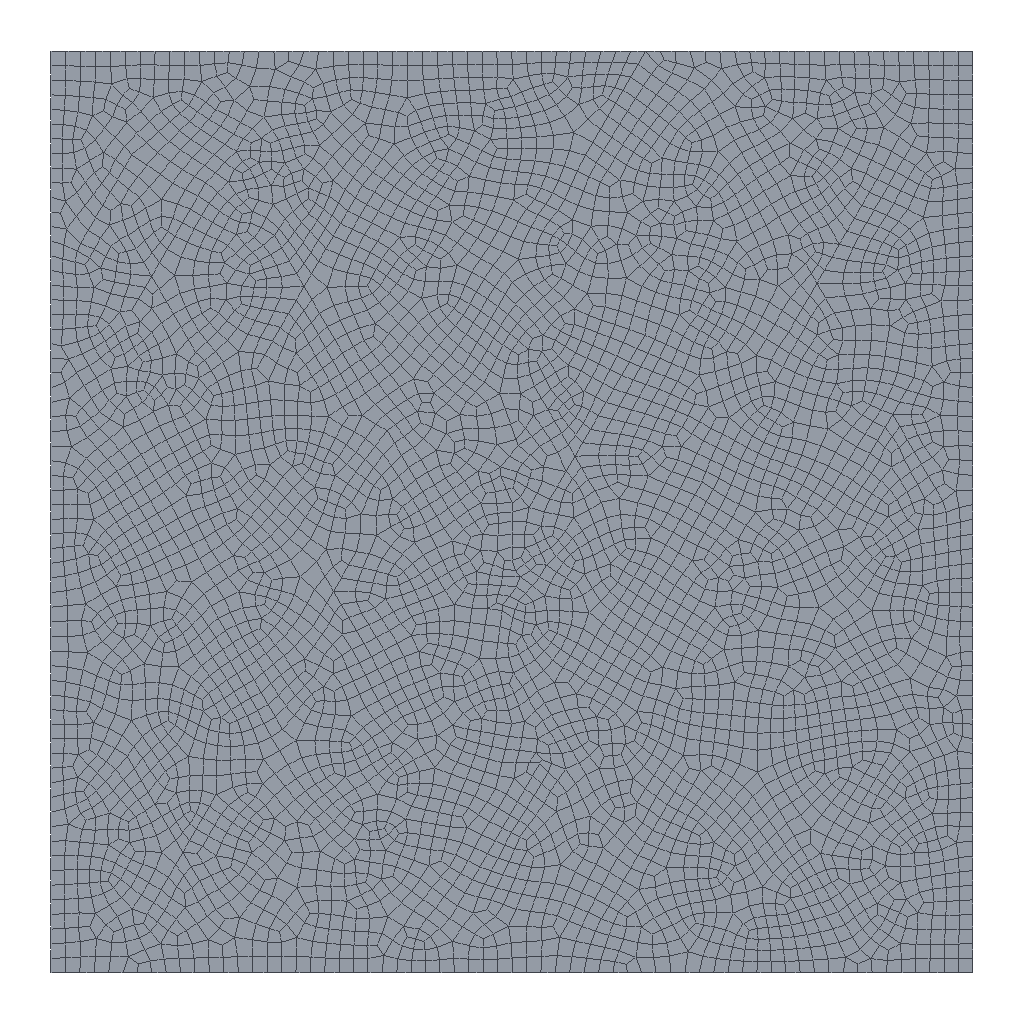Simulation study | abaqus
Notes in the study folder:
模型参数
尺寸 10cm*10cm
预制裂隙如cae
注入位置 和cae文件一样
渗透率 1e-16 m^2
孔隙度 3%
比热容 1.26 kJ/ （kg*K）
热导率 0.25 W/(m·K）
杨氏模量 3000MPa
泊松比 0.35
密度 1.3 g/cm^3

co2流体
 密度 0.5g / cm^3
 粘度 0.000026ps*s
滤失系数 10-3m/min^0.5
温度40℃


注入条件
40ml/min

加载条件
最小水平主应力 11MPa
最大水平主应力  15MPa

温度模型
骨架温度是40℃往中心传导
流体温度是40℃扩展过程中传导
Set-up summary:
category,name,step,type,value,unit,region
solver,abaqus
solver,version,,,Abaqus/Standard 3DEXPERIENCE R2017x
units,not stated in the deck,,not stated
analysis,deck,,geostatic,geostatic
load_step,Step-1,Step-1,geostatic
load_step,Step-2,Step-2,soils
load_step,requested,,,2
mesh,nodes,,,5515
mesh,elements,,,5115
element_type,CPE4RP,,plane,4799
element_type,COH2D4P,,cohesive,316
load,load commands in deck,,count,1
bc,support commands in deck,,count,2
material,MATERIAL-COHE1,,in results
material,MATERIAL-COHE2,,in results
material,MATERIAL-ROCK,,in results
check,setup vs results,,match,"per instance, exact: element labels, types and connectivity; labels of the nodes the elements use; coordinates of those nodes at SINGLE_PRECISION in 1 of 1 instance(s)"
Abaqus input file, long lists of numbers shortened:
*Heading
** Job name: Job-2 Model name: Model-2-crack
** Generated by: Abaqus/CAE 2017
*Preprint, echo=NO, model=NO, history=NO, contact=NO
**
** PARTS
**
*Part, name=Part-1
*Node
      1,   6.038,  -20.003
      2,   6.831,  -18.63
** (5513 more lines like these left out)
*Element, type=CPE4RP
   1, 1235,  227, 1736, 1684
   2, 1737, 1685, 1236,  228
** (4797 more lines like these left out)
*Element, type=COH2D4P
4800,  255, 1262, 4927,  255,  255, 5184
4801, 1262,  252, 4928, 4927, 5184, 5185
** (314 more lines like these left out)
*Nset, nset=Set-5
    1,    2,    3,    4,    5,    6,    7,    8,    9,   10,   11,   12,   13,   14,   15,   16
   17,   18,   19,   20,   21,   22,   23,   24,   25,   26,   27,   28,   29,   30,   31,   32
** (325 more lines like these left out)
*Elset, elset=Set-5, generate
    1,  4799,     1
*Elset, elset=CohesiveSeam-1-Elements, generate
 4800,  5080,     1
*Nset, nset=CohesiveSeam-1-TopNodes
    1,    2,    3,    4,    5,    6,    7,    8,    9,   10,   11,   12,   13,   14,   15,   16
   17,   18,   19,   20,   21,   22,   23,   24,   25,   26,   27,   28,   29,   30,   31,   32
** (18 more lines like these left out)
*Nset, nset=CohesiveSeam-1-BottomNodes
    4,    5,   13,   14,   15,   16,   17,   18,   22,   24,   28,   29,   33,   34,   37,   38
   39,   40,   44,   45,   47,   48,   50,   51,   52,   56,   57,   65,   66,   70,   71,   72
** (18 more lines like these left out)
*Nset, nset=CohesiveSeam-1-MidNodes
    4,    5,   13,   14,   15,   16,   17,   22,   24,   28,   29,   34,   37,   38,   40,   44
   45,   48,   50,   51,   52,   56,   57,   65,   66,   70,   71,   72,   73,   77,   78,   80
** (19 more lines like these left out)
*Elset, elset=CohesiveSeam-2-Elements, generate
 5081,  5115,     1
*Nset, nset=CohesiveSeam-2-TopNodes
  159,  160,  161,  163,  164,  165,  166,  167,  168,  169,  170,  171,  172,  173,  174,  175
  176,  177,  179,  180, 1169, 1170, 1171, 1175, 1176, 1177, 1178, 1182, 5452, 5453, 5454, 5455
** (2 more lines like these left out)
*Nset, nset=CohesiveSeam-2-BottomNodes
  160,  161,  162,  163,  165,  166,  167,  168,  169,  170,  171,  172,  173,  174,  175,  176
  177,  178,  179,  180, 1172, 1173, 1174, 1179, 1180, 1181, 5448, 5449, 5450, 5451, 5452, 5457
** (2 more lines like these left out)
*Nset, nset=CohesiveSeam-2-MidNodes
  161,  180, 5482, 5483, 5484, 5485, 5486, 5487, 5488, 5489, 5490, 5491, 5492, 5493, 5494, 5495
 5496, 5497, 5498, 5499, 5500, 5501, 5502, 5503, 5504, 5505, 5506, 5507, 5508, 5509, 5510, 5511
** (1 more lines like these left out)
*Nset, nset=inject
 5502,
*Elset, elset=initial-crack, generate
 5101,  5103,     1
*Elset, elset=__PickedSurf14_S3, internal
   61,   78,   80,  100,  103,  111,  114,  132,  145,  165,  179,  180,  181,  201,  214,  241
  283,  284,  324,  342,  343,  400,  403,  526,  533,  544,  545,  555,  568,  585,  586,  595
** (17 more lines like these left out)
*Elset, elset=__PickedSurf14_S4, internal
    6,   15,   46,   58,   65,   69,   82,   87,   88,  120,  121,  162,  173,  202,  234,  298
  311,  314,  327,  334,  353,  355,  388,  401,  421,  438,  448,  455,  458,  465,  466,  470
** (6 more lines like these left out)
*Elset, elset=__PickedSurf14_S1, internal
   55,   81,  128,  129,  130,  144,  152,  164,  199,  200,  216,  233,  242,  274,  276,  277
  322,  325,  336,  338,  339,  345,  407,  434,  495,  500,  524,  534,  543,  554,  594,  596
** (11 more lines like these left out)
*Elset, elset=__PickedSurf14_S2, internal
    7,    8,    9,   26,   28,   44,   57,   70,   83,   85,  138,  151,  170,  195,  218,  242
  243,  244,  245,  247,  267,  299,  308,  312,  333,  340,  354,  422,  437,  450,  451,  471
** (7 more lines like these left out)
*Surface, type=ELEMENT, name=_PickedSurf14, internal
__PickedSurf14_S3, S3
__PickedSurf14_S4, S4
__PickedSurf14_S2, S2
__PickedSurf14_S1, S1
*Elset, elset=__PickedSurf21_S1, internal
  885, 1494, 5081, 5082, 5083, 5084, 5085, 5091, 5092, 5093
*Elset, elset=__PickedSurf21_S3, internal
  319,  884, 1906, 5086, 5087, 5088, 5089, 5090, 5094, 5095, 5096, 5097, 5099, 5103, 5105, 5106
 5108, 5109, 5111, 5112, 5113, 5114, 5115
*Elset, elset=__PickedSurf21_S2, internal
 1898, 1905, 4579
*Elset, elset=__PickedSurf21_S4, internal
  922, 1902, 1903, 2028, 2052
*Surface, type=ELEMENT, name=_PickedSurf21, internal
__PickedSurf21_S1, S1
__PickedSurf21_S3, S3
__PickedSurf21_S2, S2
__PickedSurf21_S4, S4
*Elset, elset=_CohesiveSeam-1-TopSurf_S3, internal, generate
 4800,  5080,     1
*Surface, type=ELEMENT, name=CohesiveSeam-1-TopSurf
_CohesiveSeam-1-TopSurf_S3, S3
*Elset, elset=_CohesiveSeam-1-BottomSurf_S1, internal, generate
 4800,  5080,     1
*Surface, type=ELEMENT, name=CohesiveSeam-1-BottomSurf
_CohesiveSeam-1-BottomSurf_S1, S1
*Elset, elset=_CohesiveSeam-2-TopSurf_S3, internal, generate
 5081,  5115,     1
*Surface, type=ELEMENT, name=CohesiveSeam-2-TopSurf
_CohesiveSeam-2-TopSurf_S3, S3
*Elset, elset=_CohesiveSeam-2-BottomSurf_S1, internal, generate
 5081,  5115,     1
*Surface, type=ELEMENT, name=CohesiveSeam-2-BottomSurf
_CohesiveSeam-2-BottomSurf_S1, S1
** Section: Section-rock
*Solid Section, elset=Set-5, material=Material-rock
,
** Section: Section-cohe1
*Cohesive Section, elset=CohesiveSeam-1-Elements, controls=EC-1, material=Material-cohe1, response=TRACTION SEPARATION,
thickness=SPECIFIED
0.001,
** Section: Section-cohe2
*Cohesive Section, elset=CohesiveSeam-2-Elements, controls=EC-1, material=Material-cohe2, response=TRACTION SEPARATION,
thickness=SPECIFIED
0.001,
*Equation
2
5221, 8, 1
5224, 8, -1
*Equation
2
5224, 8, 1
5228, 8, -1
*Equation
2
5246, 8, 1
5251, 8, -1
*Equation
2
5251, 8, 1
5253, 8, -1
*Equation
2
5253, 8, 1
5257, 8, -1
*Equation
2
5266, 8, 1
5268, 8, -1
*Equation
2
5268, 8, 1
5271, 8, -1
*Equation
2
5271, 8, 1
5276, 8, -1
*Equation
2
5314, 8, 1
5317, 8, -1
*Equation
2
5317, 8, 1
5320, 8, -1
*Equation
2
5320, 8, 1
5326, 8, -1
*Equation
2
5345, 8, 1
5353, 8, -1
*Equation
2
5353, 8, 1
5357, 8, -1
*Equation
2
5357, 8, 1
5361, 8, -1
*Equation
2
5376, 8, 1
5380, 8, -1
*Equation
2
5380, 8, 1
5386, 8, -1
*Equation
2
5386, 8, 1
5394, 8, -1
*Equation
2
5417, 8, 1
5419, 8, -1
*Equation
2
5419, 8, 1
5423, 8, -1
*Equation
2
5423, 8, 1
5426, 8, -1
*End Part
**
**
** ASSEMBLY
**
*Assembly, name=Assembly
**
*Instance, name=Part-1-1, part=Part-1
*End Instance
**
*Nset, nset=Set-6, instance=Part-1-1
    1,    2,    3,    4,    5,    6,    7,    8,    9,   10,   11,   12,   13,   14,   15,   16
   17,   18,   19,   20,   21,   22,   23,   24,   25,   26,   27,   28,   29,   30,   31,   32
** (325 more lines like these left out)
*Elset, elset=Set-6, instance=Part-1-1
    1,    2,    3,    4,    5,    6,    7,    8,    9,   10,   11,   12,   13,   14,   15,   16
   17,   18,   19,   20,   21,   22,   23,   24,   25,   26,   27,   28,   29,   30,   31,   32
** (316 more lines like these left out)
*Nset, nset=Set-7, instance=Part-1-1
  181,  182,  183,  184,  185,  186,  187,  188,  189,  190,  191,  192,  193,  194,  195,  196
  197,  198,  199,  200,  201,  202,  203,  204,  205,  206,  207,  208,  209,  210,  211,  212
** (14 more lines like these left out)
*Elset, elset=Set-7, instance=Part-1-1
    1,    2,    3,   10,   49,   50,   51,   52,   53,   56,   59,   74,   75,   76,   77,   89
   90,   91,   94,   95,   97,  113,  148,  160,  209,  210,  211,  220,  222,  257,  258,  259
** (14 more lines like these left out)
*Nset, nset=Set-8, instance=Part-1-1
    1,    2,    3,    4,    5,    6,    7,    8,    9,   10,   11,   12,   13,   14,   15,   16
   17,   18,   19,   20,   21,   22,   23,   24,   25,   26,   27,   28,   29,   30,   31,   32
** (325 more lines like these left out)
*Elset, elset=Set-8, instance=Part-1-1, generate
    1,  4799,     1
*Nset, nset=Set-9, instance=Part-1-1
    1,    2,    3,    4,    5,    6,    7,    8,    9,   10,   11,   12,   13,   14,   15,   16
   17,   18,   19,   20,   21,   22,   23,   24,   25,   26,   27,   28,   29,   30,   31,   32
** (325 more lines like these left out)
*Elset, elset=Set-9, instance=Part-1-1, generate
    1,  5115,     1
*Nset, nset=Set-10, instance=Part-1-1
    1,    2,    3,    4,    5,    6,    7,    8,    9,   10,   11,   12,   13,   14,   15,   16
   17,   18,   19,   20,   21,   22,   23,   24,   25,   26,   27,   28,   29,   30,   31,   32
** (325 more lines like these left out)
*Elset, elset=Set-10, instance=Part-1-1, generate
    1,  5115,     1
*Nset, nset=Set-11, instance=Part-1-1
  210,  211,  212,  213,  214,  215,  216,  217,  218,  219,  220,  221,  222,  223,  224,  225
  226,  227,  228,  229,  230,  231,  232,  233,  234,  235,  236,  237,  238,  239,  240,  241
** (6 more lines like these left out)
*Elset, elset=Set-11, instance=Part-1-1
    1,    2,    3,   10,   94,   95,   97,  148,  160,  427,  429,  431,  517,  519,  521,  549
  551,  559,  561,  562,  583,  584,  590,  661,  663,  664,  807,  809,  811,  833,  844,  846
** (6 more lines like these left out)
*Nset, nset=Set-12, instance=Part-1-1
  181,  182,  183,  184,  185,  186,  187,  188,  189,  190,  191,  192,  193,  194,  195,  196
  197,  198,  199,  200,  201,  202,  203,  204,  205,  206,  207,  208,  209,  210,  211, 1183
** (3 more lines like these left out)
*Elset, elset=Set-12, instance=Part-1-1
   49,   50,   51,   52,   53,   56,   59,   74,   75,   76,   77,   89,   90,   91,  113,  371
  373,  642,  643,  644,  645,  942,  947,  952,  955,  959,  969,  973,  976,  977,  984,  987
** (2 more lines like these left out)
*Nset, nset=Set-13, instance=Part-1-1
    1,    2,    3,    4,    5,    6,    7,    8,    9,   10,   11,   12,   13,   14,   15,   16
   17,   18,   19,   20,   21,   22,   23,   24,   25,   26,   27,   28,   29,   30,   31,   32
** (325 more lines like these left out)
*Elset, elset=Set-13, instance=Part-1-1, generate
    1,  5115,     1
*End Assembly
**
** ELEMENT CONTROLS
**
*Section Controls, name=EC-1, ELEMENT DELETION=YES
1., 1., 1.
*Amplitude, name=Amp-1
             0.,              0.,              1.,              1.
*Amplitude, name=Amp-2
             0.,              0.,            500.,              1.
**
** MATERIALS
**
*Material, name=Material-cohe1
*Conductivity
 0.25,
*Damage Initiation, criterion=MAXS
20000.,20000.,20000.
*Damage Evolution, type=DISPLACEMENT
 1e-10,
*Density
1300.,
*Elastic, type=TRACTION
 1.5e+10, 1.5e+10, 1.5e+10
*Expansion
 6e-06,
*Fluid Leakoff
 1e-14, 1e-14
*Gap Flow
 0.001,
*Material, name=Material-cohe2
*Damage Initiation, criterion=MAXS
600000.,600000.,600000.
*Damage Evolution, type=DISPLACEMENT
 1e-12,
*Damage Stabilization
0.0001
*Density
1300.,
*Elastic, type=TRACTION
 1.5e+10, 1.5e+10, 1.5e+10
*Fluid Leakoff
 1e-14, 1e-14
*Gap Flow
 0.001,
*Material, name=Material-rock
*Conductivity
 0.25,
*Density
1300.,
*Elastic
 1.5e+10, 0.25
*Expansion
 5e-06,
*Permeability, specific=9800.
 1e-06, 0.1
*Specific Heat
1260.,
**
** PHYSICAL CONSTANTS
**
*Physical Constants, absolute zero=-273., stefan boltzmann=5.67e-08
**
** PREDEFINED FIELDS
**
** Name: Predefined Field-2   Type: Stress
*Initial Conditions, type=STRESS
Set-8, -100000., -100000., 0., 0.,
** Name: Predefined Field-3   Type: Void ratio
*Initial Conditions, TYPE=RATIO
Set-9, 0.1
** ----------------------------------------------------------------
**
*initial conditions, type=initial gap
Part-1-1.initial-crack
** STEP: Step-1
**
*Step, name=Step-1, nlgeom=YES, unsymm=YES
*Geostatic
**
** BOUNDARY CONDITIONS
**
** Name: [REDACTED] : Displacement/rotation angle
*Boundary
Set-11, 1, 1
** Name: [REDACTED] : Displacement/rotation angle
*Boundary
Set-12, 2, 2
**
** CONTROLS
**
*Controls, reset
*Controls, parameters=time incrementation
, , , , , , , 10, , ,
**
** OUTPUT REQUESTS
**
*Restart, write, frequency=0
**
** FIELD OUTPUT: F-Output-2
**
*Output, field
*Node Output
CF, CFF, NT, POR, RF, RM, RT, RVF
RVT, U, V
*Element Output, directions=YES
E, FLUVR, FLVEL, GELVR, LE, MFL, MFLT, MISES, MISESMAX, MISESONLY, PE, PEEQ, PEEQMAX, PEEQT, PEMAG, PRESSONLY
RD, S, SAT, SDEG, SF, SSAVG, TEMP, VEEQ, VOIDR, VVF, VVFG, VVFN
*Contact Output
CDISP, CSTRESS, PFL, PFLA, PTL, PTLA
**
** HISTORY OUTPUT: H-Output-2
**
*Output, history, variable=PRESELECT
*End Step
** ----------------------------------------------------------------
**
** STEP: Step-2
**
*Step, name=Step-2, nlgeom=YES, inc=10000, unsymm=YES
*Soils, consolidation, end=PERIOD, utol=1e+10, cetol=1., stabilize=0.0002, allsdtol=0.05, continue=NO
0.1, 500., 1e-05, 20.,
**
** LOADS
**
** Name: Load-1   Type: Concentrated pore fluid
*Cflow, amplitude=Amp-2
Part-1-1.inject,  , -0.002
**
** PREDEFINED FIELDS
**
** Name: Predefined Field-TT   Type: Temperature
*Temperature, file=D:\_______________\_____\________._______________________________________
**
** OUTPUT REQUESTS
**
*Restart, write, frequency=0
**
** FIELD OUTPUT: F-Output-2
**
*Output, field
*Node Output
CF, CFF, NT, POR, RF, RM, RT, RVF
RVT, U, V
*Element Output, directions=YES
E, FLUVR, FLVEL, GELVR, LE, MISES, MISESMAX, MISESONLY, PE, PEEQ, PEEQMAX, PEEQT, PEMAG, PRESSONLY, RD, S
SAT, SDEG, SF, SSAVG, TEMP, VEEQ, VOIDR, VVF, VVFG, VVFN,pfopen
*Contact Output
CDISP, CSTRESS, PFL, PFLA, PTL, PTLA
**
** HISTORY OUTPUT: H-Output-2
**
*Output, history, variable=PRESELECT
*End Step
Results summary:
result,step,,completed,increments=1 time=1.0/1.0
result,step,,completed,increments=85 time=500.0/500.0
result,analysis,,,"soils, consolidation"
result,last_loadstep,,,2
result,primary field,,,"U, POR"
result,reaction total,,FX,-1596.375,model units
result,reaction total,,FY,196035.179,model units
result,reaction total,,FZ,0.0,model units